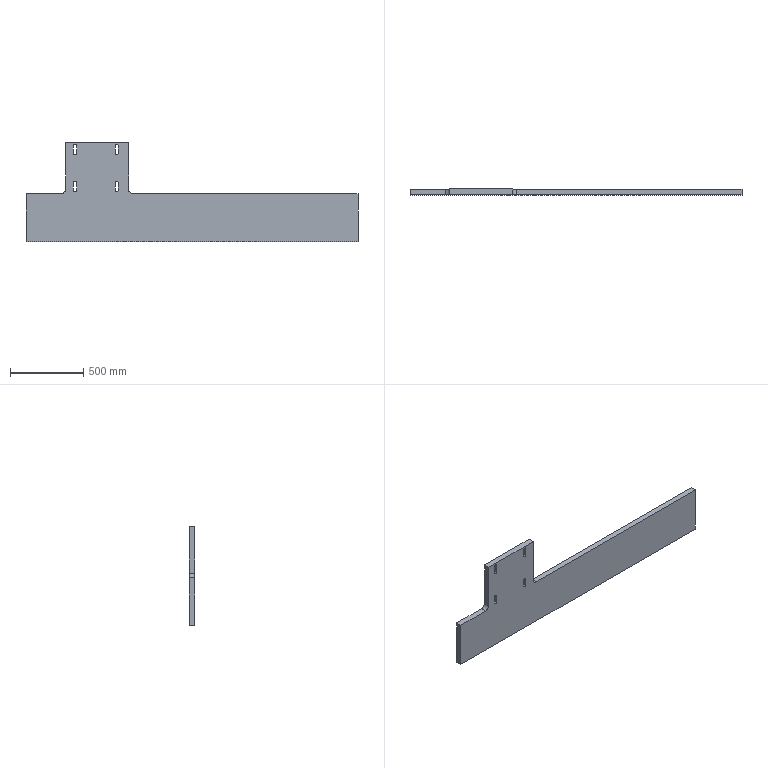Part | SolidWorks | features Cut 1, Extrusion 1, Fillet 1, ICE 1 | 1 solid | 32 faces | box 2266 x 40 x 677.5 mm | volume 35483230 mm3 | plane 18 | cylinder 14 | commonest cylinder face diameters 22 x12 60 x2
STEP:
#1=CARTESIAN_POINT('',(-514.,0.,500.75));
#2=VERTEX_POINT('',#1);
#3=CARTESIAN_POINT('',(-503.,0.,489.75));
#4=VERTEX_POINT('',#3);
#5=CARTESIAN_POINT('',(-514.,0.,489.75));
#6=DIRECTION('',(0.,1.,0.));
#7=DIRECTION('',(0.,0.,1.));
#8=AXIS2_PLACEMENT_3D('',#5,#6,#7);
#9=CIRCLE('',#8,11.);
#10=EDGE_CURVE('',#2,#4,#9,.T.);
#11=ORIENTED_EDGE('',*,*,#10,.F.);
#12=CARTESIAN_POINT('',(-514.,40.,500.75));
#13=VERTEX_POINT('',#12);
#14=CARTESIAN_POINT('',(-514.,0.,500.75));
#15=DIRECTION('',(0.,1.,0.));
#16=VECTOR('',#15,1000.);
#17=LINE('',#14,#16);
#18=EDGE_CURVE('',#2,#13,#17,.T.);
#19=ORIENTED_EDGE('',*,*,#18,.T.);
#20=CARTESIAN_POINT('',(-503.,40.,489.75));
#21=VERTEX_POINT('',#20);
#22=CARTESIAN_POINT('',(-514.,40.,489.75));
#23=DIRECTION('',(0.,1.,0.));
#24=DIRECTION('',(0.,0.,1.));
#25=AXIS2_PLACEMENT_3D('',#22,#23,#24);
#26=CIRCLE('',#25,11.);
#27=EDGE_CURVE('',#13,#21,#26,.T.);
#28=ORIENTED_EDGE('',*,*,#27,.T.);
#29=CARTESIAN_POINT('',(-503.,0.,489.75));
#30=DIRECTION('',(0.,1.,0.));
#31=VECTOR('',#30,1000.);
#32=LINE('',#29,#31);
#33=EDGE_CURVE('',#4,#21,#32,.T.);
#34=ORIENTED_EDGE('',*,*,#33,.F.);
#35=EDGE_LOOP('',(#11,#19,#28,#34));
#36=FACE_OUTER_BOUND('',#35,.T.);
#37=CARTESIAN_POINT('',(-514.,0.,489.75));
#38=DIRECTION('',(0.,1.,0.));
#39=DIRECTION('',(0.,0.,1.));
#40=AXIS2_PLACEMENT_3D('',#37,#38,#39);
#41=CYLINDRICAL_SURFACE('',#40,11.);
#42=ADVANCED_FACE('',(#36),#41,.F.);
#43=CARTESIAN_POINT('',(-798.,0.,248.75));
#44=VERTEX_POINT('',#43);
#45=CARTESIAN_POINT('',(-787.,0.,237.75));
#46=VERTEX_POINT('',#45);
#47=CARTESIAN_POINT('',(-798.,0.,237.75));
#48=DIRECTION('',(0.,1.,0.));
#49=DIRECTION('',(0.,0.,1.));
#50=AXIS2_PLACEMENT_3D('',#47,#48,#49);
#51=CIRCLE('',#50,11.);
#52=EDGE_CURVE('',#44,#46,#51,.T.);
#53=ORIENTED_EDGE('',*,*,#52,.F.);
#54=CARTESIAN_POINT('',(-798.,40.,248.75));
#55=VERTEX_POINT('',#54);
#56=CARTESIAN_POINT('',(-798.,0.,248.75));
#57=DIRECTION('',(0.,1.,0.));
#58=VECTOR('',#57,1000.);
#59=LINE('',#56,#58);
#60=EDGE_CURVE('',#44,#55,#59,.T.);
#61=ORIENTED_EDGE('',*,*,#60,.T.);
#62=CARTESIAN_POINT('',(-787.,40.,237.75));
#63=VERTEX_POINT('',#62);
#64=CARTESIAN_POINT('',(-798.,40.,237.75));
#65=DIRECTION('',(0.,1.,0.));
#66=DIRECTION('',(0.,0.,1.));
#67=AXIS2_PLACEMENT_3D('',#64,#65,#66);
#68=CIRCLE('',#67,11.);
#69=EDGE_CURVE('',#55,#63,#68,.T.);
#70=ORIENTED_EDGE('',*,*,#69,.T.);
#71=CARTESIAN_POINT('',(-787.,0.,237.75));
#72=DIRECTION('',(0.,1.,0.));
#73=VECTOR('',#72,1000.);
#74=LINE('',#71,#73);
#75=EDGE_CURVE('',#46,#63,#74,.T.);
#76=ORIENTED_EDGE('',*,*,#75,.F.);
#77=EDGE_LOOP('',(#53,#61,#70,#76));
#78=FACE_OUTER_BOUND('',#77,.T.);
#79=CARTESIAN_POINT('',(-798.,0.,237.75));
#80=DIRECTION('',(0.,1.,0.));
#81=DIRECTION('',(0.,0.,1.));
#82=AXIS2_PLACEMENT_3D('',#79,#80,#81);
#83=CYLINDRICAL_SURFACE('',#82,11.);
#84=ADVANCED_FACE('',(#78),#83,.F.);
#85=CARTESIAN_POINT('',(-798.,0.,500.75));
#86=VERTEX_POINT('',#85);
#87=CARTESIAN_POINT('',(-787.,0.,489.75));
#88=VERTEX_POINT('',#87);
#89=CARTESIAN_POINT('',(-798.,0.,489.75));
#90=DIRECTION('',(0.,1.,0.));
#91=DIRECTION('',(0.,0.,1.));
#92=AXIS2_PLACEMENT_3D('',#89,#90,#91);
#93=CIRCLE('',#92,11.);
#94=EDGE_CURVE('',#86,#88,#93,.T.);
#95=ORIENTED_EDGE('',*,*,#94,.F.);
#96=CARTESIAN_POINT('',(-798.,40.,500.75));
#97=VERTEX_POINT('',#96);
#98=CARTESIAN_POINT('',(-798.,0.,500.75));
#99=DIRECTION('',(0.,1.,0.));
#100=VECTOR('',#99,1000.);
#101=LINE('',#98,#100);
#102=EDGE_CURVE('',#86,#97,#101,.T.);
#103=ORIENTED_EDGE('',*,*,#102,.T.);
#104=CARTESIAN_POINT('',(-787.,40.,489.75));
#105=VERTEX_POINT('',#104);
#106=CARTESIAN_POINT('',(-798.,40.,489.75));
#107=DIRECTION('',(0.,1.,0.));
#108=DIRECTION('',(0.,0.,1.));
#109=AXIS2_PLACEMENT_3D('',#106,#107,#108);
#110=CIRCLE('',#109,11.);
#111=EDGE_CURVE('',#97,#105,#110,.T.);
#112=ORIENTED_EDGE('',*,*,#111,.T.);
#113=CARTESIAN_POINT('',(-787.,0.,489.75));
#114=DIRECTION('',(0.,1.,0.));
#115=VECTOR('',#114,1000.);
#116=LINE('',#113,#115);
#117=EDGE_CURVE('',#88,#105,#116,.T.);
#118=ORIENTED_EDGE('',*,*,#117,.F.);
#119=EDGE_LOOP('',(#95,#103,#112,#118));
#120=FACE_OUTER_BOUND('',#119,.T.);
#121=CARTESIAN_POINT('',(-798.,0.,489.75));
#122=DIRECTION('',(0.,1.,0.));
#123=DIRECTION('',(0.,0.,1.));
#124=AXIS2_PLACEMENT_3D('',#121,#122,#123);
#125=CYLINDRICAL_SURFACE('',#124,11.);
#126=ADVANCED_FACE('',(#120),#125,.F.);
#127=CARTESIAN_POINT('',(-514.,0.,248.75));
#128=VERTEX_POINT('',#127);
#129=CARTESIAN_POINT('',(-503.,0.,237.75));
#130=VERTEX_POINT('',#129);
#131=CARTESIAN_POINT('',(-514.,0.,237.75));
#132=DIRECTION('',(0.,1.,0.));
#133=DIRECTION('',(0.,0.,1.));
#134=AXIS2_PLACEMENT_3D('',#131,#132,#133);
#135=CIRCLE('',#134,11.);
#136=EDGE_CURVE('',#128,#130,#135,.T.);
#137=ORIENTED_EDGE('',*,*,#136,.F.);
#138=CARTESIAN_POINT('',(-514.,40.,248.75));
#139=VERTEX_POINT('',#138);
#140=CARTESIAN_POINT('',(-514.,0.,248.75));
#141=DIRECTION('',(0.,1.,0.));
#142=VECTOR('',#141,1000.);
#143=LINE('',#140,#142);
#144=EDGE_CURVE('',#128,#139,#143,.T.);
#145=ORIENTED_EDGE('',*,*,#144,.T.);
#146=CARTESIAN_POINT('',(-503.,40.,237.75));
#147=VERTEX_POINT('',#146);
#148=CARTESIAN_POINT('',(-514.,40.,237.75));
#149=DIRECTION('',(0.,1.,0.));
#150=DIRECTION('',(0.,0.,1.));
#151=AXIS2_PLACEMENT_3D('',#148,#149,#150);
#152=CIRCLE('',#151,11.);
#153=EDGE_CURVE('',#139,#147,#152,.T.);
#154=ORIENTED_EDGE('',*,*,#153,.T.);
#155=CARTESIAN_POINT('',(-503.,0.,237.75));
#156=DIRECTION('',(0.,1.,0.));
#157=VECTOR('',#156,1000.);
#158=LINE('',#155,#157);
#159=EDGE_CURVE('',#130,#147,#158,.T.);
#160=ORIENTED_EDGE('',*,*,#159,.F.);
#161=EDGE_LOOP('',(#137,#145,#154,#160));
#162=FACE_OUTER_BOUND('',#161,.T.);
#163=CARTESIAN_POINT('',(-514.,0.,237.75));
#164=DIRECTION('',(0.,1.,0.));
#165=DIRECTION('',(0.,0.,1.));
#166=AXIS2_PLACEMENT_3D('',#163,#164,#165);
#167=CYLINDRICAL_SURFACE('',#166,11.);
#168=ADVANCED_FACE('',(#162),#167,.F.);
#169=CARTESIAN_POINT('',(-403.,40.,163.75));
#170=VERTEX_POINT('',#169);
#171=CARTESIAN_POINT('',(1133.,40.,163.75));
#172=VERTEX_POINT('',#171);
#173=CARTESIAN_POINT('',(-1133.,40.,163.75));
#174=DIRECTION('',(1.,0.,0.));
#175=VECTOR('',#174,1000.);
#176=LINE('',#173,#175);
#177=EDGE_CURVE('',#170,#172,#176,.T.);
#178=ORIENTED_EDGE('',*,*,#177,.F.);
#179=CARTESIAN_POINT('',(-403.,0.,163.75));
#180=VERTEX_POINT('',#179);
#181=CARTESIAN_POINT('',(-403.,40.,163.75));
#182=DIRECTION('',(0.,-1.,0.));
#183=VECTOR('',#182,1000.);
#184=LINE('',#181,#183);
#185=EDGE_CURVE('',#170,#180,#184,.T.);
#186=ORIENTED_EDGE('',*,*,#185,.T.);
#187=CARTESIAN_POINT('',(1133.,0.,163.75));
#188=VERTEX_POINT('',#187);
#189=CARTESIAN_POINT('',(-1133.,0.,163.75));
#190=DIRECTION('',(1.,0.,0.));
#191=VECTOR('',#190,1000.);
#192=LINE('',#189,#191);
#193=EDGE_CURVE('',#180,#188,#192,.T.);
#194=ORIENTED_EDGE('',*,*,#193,.T.);
#195=CARTESIAN_POINT('',(1133.,40.,163.75));
#196=DIRECTION('',(0.,-1.,0.));
#197=VECTOR('',#196,1000.);
#198=LINE('',#195,#197);
#199=EDGE_CURVE('',#172,#188,#198,.T.);
#200=ORIENTED_EDGE('',*,*,#199,.F.);
#201=EDGE_LOOP('',(#178,#186,#194,#200));
#202=FACE_OUTER_BOUND('',#201,.T.);
#203=CARTESIAN_POINT('',(-1133.,40.,163.75));
#204=DIRECTION('',(0.,0.,-1.));
#205=DIRECTION('',(-1.,0.,0.));
#206=AXIS2_PLACEMENT_3D('',#203,#204,#205);
#207=PLANE('',#206);
#208=ADVANCED_FACE('',(#202),#207,.F.);
#209=CARTESIAN_POINT('',(1133.,0.,-163.75));
#210=VERTEX_POINT('',#209);
#211=CARTESIAN_POINT('',(1133.,0.,163.75));
#212=DIRECTION('',(0.,0.,-1.));
#213=VECTOR('',#212,1000.);
#214=LINE('',#211,#213);
#215=EDGE_CURVE('',#188,#210,#214,.T.);
#216=ORIENTED_EDGE('',*,*,#215,.T.);
#217=CARTESIAN_POINT('',(1133.,40.,-163.75));
#218=VERTEX_POINT('',#217);
#219=CARTESIAN_POINT('',(1133.,40.,-163.75));
#220=DIRECTION('',(0.,-1.,0.));
#221=VECTOR('',#220,1000.);
#222=LINE('',#219,#221);
#223=EDGE_CURVE('',#218,#210,#222,.T.);
#224=ORIENTED_EDGE('',*,*,#223,.F.);
#225=CARTESIAN_POINT('',(1133.,40.,163.75));
#226=DIRECTION('',(0.,0.,-1.));
#227=VECTOR('',#226,1000.);
#228=LINE('',#225,#227);
#229=EDGE_CURVE('',#172,#218,#228,.T.);
#230=ORIENTED_EDGE('',*,*,#229,.F.);
#231=ORIENTED_EDGE('',*,*,#199,.T.);
#232=EDGE_LOOP('',(#216,#224,#230,#231));
#233=FACE_OUTER_BOUND('',#232,.T.);
#234=CARTESIAN_POINT('',(1133.,40.,163.75));
#235=DIRECTION('',(-1.,0.,0.));
#236=DIRECTION('',(0.,0.,1.));
#237=AXIS2_PLACEMENT_3D('',#234,#235,#236);
#238=PLANE('',#237);
#239=ADVANCED_FACE('',(#233),#238,.F.);
#240=CARTESIAN_POINT('',(-1133.,0.,-163.75));
#241=VERTEX_POINT('',#240);
#242=CARTESIAN_POINT('',(-1133.,0.,-163.75));
#243=DIRECTION('',(-1.,0.,0.));
#244=VECTOR('',#243,1000.);
#245=LINE('',#242,#244);
#246=EDGE_CURVE('',#210,#241,#245,.T.);
#247=ORIENTED_EDGE('',*,*,#246,.T.);
#248=CARTESIAN_POINT('',(-1133.,40.,-163.75));
#249=VERTEX_POINT('',#248);
#250=CARTESIAN_POINT('',(-1133.,40.,-163.75));
#251=DIRECTION('',(0.,-1.,0.));
#252=VECTOR('',#251,1000.);
#253=LINE('',#250,#252);
#254=EDGE_CURVE('',#249,#241,#253,.T.);
#255=ORIENTED_EDGE('',*,*,#254,.F.);
#256=CARTESIAN_POINT('',(-1133.,40.,-163.75));
#257=DIRECTION('',(-1.,0.,0.));
#258=VECTOR('',#257,1000.);
#259=LINE('',#256,#258);
#260=EDGE_CURVE('',#218,#249,#259,.T.);
#261=ORIENTED_EDGE('',*,*,#260,.F.);
#262=ORIENTED_EDGE('',*,*,#223,.T.);
#263=EDGE_LOOP('',(#247,#255,#261,#262));
#264=FACE_OUTER_BOUND('',#263,.T.);
#265=CARTESIAN_POINT('',(-1133.,40.,-163.75));
#266=DIRECTION('',(0.,0.,1.));
#267=DIRECTION('',(1.,0.,0.));
#268=AXIS2_PLACEMENT_3D('',#265,#266,#267);
#269=PLANE('',#268);
#270=ADVANCED_FACE('',(#264),#269,.F.);
#271=CARTESIAN_POINT('',(-1133.,0.,163.75));
#272=VERTEX_POINT('',#271);
#273=CARTESIAN_POINT('',(-1133.,0.,163.75));
#274=DIRECTION('',(0.,0.,1.));
#275=VECTOR('',#274,1000.);
#276=LINE('',#273,#275);
#277=EDGE_CURVE('',#241,#272,#276,.T.);
#278=ORIENTED_EDGE('',*,*,#277,.T.);
#279=CARTESIAN_POINT('',(-1133.,40.,163.75));
#280=VERTEX_POINT('',#279);
#281=CARTESIAN_POINT('',(-1133.,40.,163.75));
#282=DIRECTION('',(0.,-1.,0.));
#283=VECTOR('',#282,1000.);
#284=LINE('',#281,#283);
#285=EDGE_CURVE('',#280,#272,#284,.T.);
#286=ORIENTED_EDGE('',*,*,#285,.F.);
#287=CARTESIAN_POINT('',(-1133.,40.,163.75));
#288=DIRECTION('',(0.,0.,1.));
#289=VECTOR('',#288,1000.);
#290=LINE('',#287,#289);
#291=EDGE_CURVE('',#249,#280,#290,.T.);
#292=ORIENTED_EDGE('',*,*,#291,.F.);
#293=ORIENTED_EDGE('',*,*,#254,.T.);
#294=EDGE_LOOP('',(#278,#286,#292,#293));
#295=FACE_OUTER_BOUND('',#294,.T.);
#296=CARTESIAN_POINT('',(-1133.,40.,163.75));
#297=DIRECTION('',(1.,0.,0.));
#298=DIRECTION('',(0.,0.,-1.));
#299=AXIS2_PLACEMENT_3D('',#296,#297,#298);
#300=PLANE('',#299);
#301=ADVANCED_FACE('',(#295),#300,.F.);
#302=CARTESIAN_POINT('',(-893.,0.,163.75));
#303=VERTEX_POINT('',#302);
#304=CARTESIAN_POINT('',(-1133.,0.,163.75));
#305=DIRECTION('',(1.,0.,0.));
#306=VECTOR('',#305,1000.);
#307=LINE('',#304,#306);
#308=EDGE_CURVE('',#272,#303,#307,.T.);
#309=ORIENTED_EDGE('',*,*,#308,.T.);
#310=CARTESIAN_POINT('',(-893.,40.,163.75));
#311=VERTEX_POINT('',#310);
#312=CARTESIAN_POINT('',(-893.,40.,163.75));
#313=DIRECTION('',(0.,1.,0.));
#314=VECTOR('',#313,1000.);
#315=LINE('',#312,#314);
#316=EDGE_CURVE('',#303,#311,#315,.T.);
#317=ORIENTED_EDGE('',*,*,#316,.T.);
#318=CARTESIAN_POINT('',(-1133.,40.,163.75));
#319=DIRECTION('',(1.,0.,0.));
#320=VECTOR('',#319,1000.);
#321=LINE('',#318,#320);
#322=EDGE_CURVE('',#280,#311,#321,.T.);
#323=ORIENTED_EDGE('',*,*,#322,.F.);
#324=ORIENTED_EDGE('',*,*,#285,.T.);
#325=EDGE_LOOP('',(#309,#317,#323,#324));
#326=FACE_OUTER_BOUND('',#325,.T.);
#327=CARTESIAN_POINT('',(-1133.,40.,163.75));
#328=DIRECTION('',(0.,0.,-1.));
#329=DIRECTION('',(-1.,0.,0.));
#330=AXIS2_PLACEMENT_3D('',#327,#328,#329);
#331=PLANE('',#330);
#332=ADVANCED_FACE('',(#326),#331,.F.);
#333=CARTESIAN_POINT('',(-525.,40.,439.75));
#334=VERTEX_POINT('',#333);
#335=CARTESIAN_POINT('',(-525.,40.,489.75));
#336=VERTEX_POINT('',#335);
#337=CARTESIAN_POINT('',(-525.,40.,439.75));
#338=DIRECTION('',(0.,0.,1.));
#339=VECTOR('',#338,1000.);
#340=LINE('',#337,#339);
#341=EDGE_CURVE('',#334,#336,#340,.T.);
#342=ORIENTED_EDGE('',*,*,#341,.F.);
#343=CARTESIAN_POINT('',(-503.,40.,439.75));
#344=VERTEX_POINT('',#343);
#345=CARTESIAN_POINT('',(-514.,40.,439.75));
#346=DIRECTION('',(0.,1.,0.));
#347=DIRECTION('',(0.,0.,1.));
#348=AXIS2_PLACEMENT_3D('',#345,#346,#347);
#349=CIRCLE('',#348,11.);
#350=EDGE_CURVE('',#344,#334,#349,.T.);
#351=ORIENTED_EDGE('',*,*,#350,.F.);
#352=CARTESIAN_POINT('',(-503.,40.,439.75));
#353=DIRECTION('',(0.,0.,-1.));
#354=VECTOR('',#353,1000.);
#355=LINE('',#352,#354);
#356=EDGE_CURVE('',#21,#344,#355,.T.);
#357=ORIENTED_EDGE('',*,*,#356,.F.);
#358=ORIENTED_EDGE('',*,*,#27,.F.);
#359=CARTESIAN_POINT('',(-514.,40.,489.75));
#360=DIRECTION('',(0.,1.,0.));
#361=DIRECTION('',(0.,0.,1.));
#362=AXIS2_PLACEMENT_3D('',#359,#360,#361);
#363=CIRCLE('',#362,11.);
#364=EDGE_CURVE('',#336,#13,#363,.T.);
#365=ORIENTED_EDGE('',*,*,#364,.F.);
#366=EDGE_LOOP('',(#342,#351,#357,#358,#365));
#367=FACE_BOUND('',#366,.T.);
#368=CARTESIAN_POINT('',(-809.,40.,187.75));
#369=VERTEX_POINT('',#368);
#370=CARTESIAN_POINT('',(-809.,40.,237.75));
#371=VERTEX_POINT('',#370);
#372=CARTESIAN_POINT('',(-809.,40.,187.75));
#373=DIRECTION('',(0.,0.,1.));
#374=VECTOR('',#373,1000.);
#375=LINE('',#372,#374);
#376=EDGE_CURVE('',#369,#371,#375,.T.);
#377=ORIENTED_EDGE('',*,*,#376,.F.);
#378=CARTESIAN_POINT('',(-787.,40.,187.75));
#379=VERTEX_POINT('',#378);
#380=CARTESIAN_POINT('',(-798.,40.,187.75));
#381=DIRECTION('',(0.,1.,0.));
#382=DIRECTION('',(0.,0.,1.));
#383=AXIS2_PLACEMENT_3D('',#380,#381,#382);
#384=CIRCLE('',#383,11.);
#385=EDGE_CURVE('',#379,#369,#384,.T.);
#386=ORIENTED_EDGE('',*,*,#385,.F.);
#387=CARTESIAN_POINT('',(-787.,40.,187.75));
#388=DIRECTION('',(0.,0.,-1.));
#389=VECTOR('',#388,1000.);
#390=LINE('',#387,#389);
#391=EDGE_CURVE('',#63,#379,#390,.T.);
#392=ORIENTED_EDGE('',*,*,#391,.F.);
#393=ORIENTED_EDGE('',*,*,#69,.F.);
#394=CARTESIAN_POINT('',(-798.,40.,237.75));
#395=DIRECTION('',(0.,1.,0.));
#396=DIRECTION('',(0.,0.,1.));
#397=AXIS2_PLACEMENT_3D('',#394,#395,#396);
#398=CIRCLE('',#397,11.);
#399=EDGE_CURVE('',#371,#55,#398,.T.);
#400=ORIENTED_EDGE('',*,*,#399,.F.);
#401=EDGE_LOOP('',(#377,#386,#392,#393,#400));
#402=FACE_BOUND('',#401,.T.);
#403=CARTESIAN_POINT('',(-809.,40.,439.75));
#404=VERTEX_POINT('',#403);
#405=CARTESIAN_POINT('',(-809.,40.,489.75));
#406=VERTEX_POINT('',#405);
#407=CARTESIAN_POINT('',(-809.,40.,439.75));
#408=DIRECTION('',(0.,0.,1.));
#409=VECTOR('',#408,1000.);
#410=LINE('',#407,#409);
#411=EDGE_CURVE('',#404,#406,#410,.T.);
#412=ORIENTED_EDGE('',*,*,#411,.F.);
#413=CARTESIAN_POINT('',(-787.,40.,439.75));
#414=VERTEX_POINT('',#413);
#415=CARTESIAN_POINT('',(-798.,40.,439.75));
#416=DIRECTION('',(0.,1.,0.));
#417=DIRECTION('',(0.,0.,1.));
#418=AXIS2_PLACEMENT_3D('',#415,#416,#417);
#419=CIRCLE('',#418,11.);
#420=EDGE_CURVE('',#414,#404,#419,.T.);
#421=ORIENTED_EDGE('',*,*,#420,.F.);
#422=CARTESIAN_POINT('',(-787.,40.,439.75));
#423=DIRECTION('',(0.,0.,-1.));
#424=VECTOR('',#423,1000.);
#425=LINE('',#422,#424);
#426=EDGE_CURVE('',#105,#414,#425,.T.);
#427=ORIENTED_EDGE('',*,*,#426,.F.);
#428=ORIENTED_EDGE('',*,*,#111,.F.);
#429=CARTESIAN_POINT('',(-798.,40.,489.75));
#430=DIRECTION('',(0.,1.,0.));
#431=DIRECTION('',(0.,0.,1.));
#432=AXIS2_PLACEMENT_3D('',#429,#430,#431);
#433=CIRCLE('',#432,11.);
#434=EDGE_CURVE('',#406,#97,#433,.T.);
#435=ORIENTED_EDGE('',*,*,#434,.F.);
#436=EDGE_LOOP('',(#412,#421,#427,#428,#435));
#437=FACE_BOUND('',#436,.T.);
#438=CARTESIAN_POINT('',(-525.,40.,187.75));
#439=VERTEX_POINT('',#438);
#440=CARTESIAN_POINT('',(-525.,40.,237.75));
#441=VERTEX_POINT('',#440);
#442=CARTESIAN_POINT('',(-525.,40.,187.75));
#443=DIRECTION('',(0.,0.,1.));
#444=VECTOR('',#443,1000.);
#445=LINE('',#442,#444);
#446=EDGE_CURVE('',#439,#441,#445,.T.);
#447=ORIENTED_EDGE('',*,*,#446,.F.);
#448=CARTESIAN_POINT('',(-503.,40.,187.75));
#449=VERTEX_POINT('',#448);
#450=CARTESIAN_POINT('',(-514.,40.,187.75));
#451=DIRECTION('',(0.,1.,0.));
#452=DIRECTION('',(0.,0.,1.));
#453=AXIS2_PLACEMENT_3D('',#450,#451,#452);
#454=CIRCLE('',#453,11.);
#455=EDGE_CURVE('',#449,#439,#454,.T.);
#456=ORIENTED_EDGE('',*,*,#455,.F.);
#457=CARTESIAN_POINT('',(-503.,40.,187.75));
#458=DIRECTION('',(0.,0.,-1.));
#459=VECTOR('',#458,1000.);
#460=LINE('',#457,#459);
#461=EDGE_CURVE('',#147,#449,#460,.T.);
#462=ORIENTED_EDGE('',*,*,#461,.F.);
#463=ORIENTED_EDGE('',*,*,#153,.F.);
#464=CARTESIAN_POINT('',(-514.,40.,237.75));
#465=DIRECTION('',(0.,1.,0.));
#466=DIRECTION('',(0.,0.,1.));
#467=AXIS2_PLACEMENT_3D('',#464,#465,#466);
#468=CIRCLE('',#467,11.);
#469=EDGE_CURVE('',#441,#139,#468,.T.);
#470=ORIENTED_EDGE('',*,*,#469,.F.);
#471=EDGE_LOOP('',(#447,#456,#462,#463,#470));
#472=FACE_BOUND('',#471,.T.);
#473=ORIENTED_EDGE('',*,*,#229,.T.);
#474=ORIENTED_EDGE('',*,*,#260,.T.);
#475=ORIENTED_EDGE('',*,*,#291,.T.);
#476=ORIENTED_EDGE('',*,*,#322,.T.);
#477=CARTESIAN_POINT('',(-863.,40.,193.75));
#478=VERTEX_POINT('',#477);
#479=CARTESIAN_POINT('',(-893.,40.,193.75));
#480=DIRECTION('',(0.,-1.,0.));
#481=DIRECTION('',(0.,0.,-1.));
#482=AXIS2_PLACEMENT_3D('',#479,#480,#481);
#483=CIRCLE('',#482,30.);
#484=EDGE_CURVE('',#311,#478,#483,.T.);
#485=ORIENTED_EDGE('',*,*,#484,.T.);
#486=CARTESIAN_POINT('',(-863.,40.,513.75));
#487=VERTEX_POINT('',#486);
#488=CARTESIAN_POINT('',(-863.,40.,163.75));
#489=DIRECTION('',(0.,0.,1.));
#490=VECTOR('',#489,1000.);
#491=LINE('',#488,#490);
#492=EDGE_CURVE('',#478,#487,#491,.T.);
#493=ORIENTED_EDGE('',*,*,#492,.T.);
#494=CARTESIAN_POINT('',(-433.,40.,513.75));
#495=VERTEX_POINT('',#494);
#496=CARTESIAN_POINT('',(-433.,40.,513.75));
#497=DIRECTION('',(1.,0.,0.));
#498=VECTOR('',#497,1000.);
#499=LINE('',#496,#498);
#500=EDGE_CURVE('',#487,#495,#499,.T.);
#501=ORIENTED_EDGE('',*,*,#500,.T.);
#502=CARTESIAN_POINT('',(-433.,40.,193.75));
#503=VERTEX_POINT('',#502);
#504=CARTESIAN_POINT('',(-433.,40.,163.75));
#505=DIRECTION('',(0.,0.,-1.));
#506=VECTOR('',#505,1000.);
#507=LINE('',#504,#506);
#508=EDGE_CURVE('',#495,#503,#507,.T.);
#509=ORIENTED_EDGE('',*,*,#508,.T.);
#510=CARTESIAN_POINT('',(-403.,40.,193.75));
#511=DIRECTION('',(0.,-1.,0.));
#512=DIRECTION('',(0.,0.,-1.));
#513=AXIS2_PLACEMENT_3D('',#510,#511,#512);
#514=CIRCLE('',#513,30.);
#515=EDGE_CURVE('',#503,#170,#514,.T.);
#516=ORIENTED_EDGE('',*,*,#515,.T.);
#517=ORIENTED_EDGE('',*,*,#177,.T.);
#518=EDGE_LOOP('',(#473,#474,#475,#476,#485,#493,#501,#509,#516,#517));
#519=FACE_OUTER_BOUND('',#518,.T.);
#520=CARTESIAN_POINT('',(0.,40.,0.));
#521=DIRECTION('',(0.,-1.,0.));
#522=DIRECTION('',(0.,0.,-1.));
#523=AXIS2_PLACEMENT_3D('',#520,#521,#522);
#524=PLANE('',#523);
#525=ADVANCED_FACE('',(#367,#402,#437,#472,#519),#524,.F.);
#526=CARTESIAN_POINT('',(-503.,0.,439.75));
#527=VERTEX_POINT('',#526);
#528=CARTESIAN_POINT('',(-525.,0.,439.75));
#529=VERTEX_POINT('',#528);
#530=CARTESIAN_POINT('',(-514.,0.,439.75));
#531=DIRECTION('',(0.,1.,0.));
#532=DIRECTION('',(0.,0.,1.));
#533=AXIS2_PLACEMENT_3D('',#530,#531,#532);
#534=CIRCLE('',#533,11.);
#535=EDGE_CURVE('',#527,#529,#534,.T.);
#536=ORIENTED_EDGE('',*,*,#535,.T.);
#537=CARTESIAN_POINT('',(-525.,0.,489.75));
#538=VERTEX_POINT('',#537);
#539=CARTESIAN_POINT('',(-525.,0.,439.75));
#540=DIRECTION('',(0.,0.,1.));
#541=VECTOR('',#540,1000.);
#542=LINE('',#539,#541);
#543=EDGE_CURVE('',#529,#538,#542,.T.);
#544=ORIENTED_EDGE('',*,*,#543,.T.);
#545=CARTESIAN_POINT('',(-514.,0.,489.75));
#546=DIRECTION('',(0.,1.,0.));
#547=DIRECTION('',(0.,0.,1.));
#548=AXIS2_PLACEMENT_3D('',#545,#546,#547);
#549=CIRCLE('',#548,11.);
#550=EDGE_CURVE('',#538,#2,#549,.T.);
#551=ORIENTED_EDGE('',*,*,#550,.T.);
#552=ORIENTED_EDGE('',*,*,#10,.T.);
#553=CARTESIAN_POINT('',(-503.,0.,439.75));
#554=DIRECTION('',(0.,0.,-1.));
#555=VECTOR('',#554,1000.);
#556=LINE('',#553,#555);
#557=EDGE_CURVE('',#4,#527,#556,.T.);
#558=ORIENTED_EDGE('',*,*,#557,.T.);
#559=EDGE_LOOP('',(#536,#544,#551,#552,#558));
#560=FACE_BOUND('',#559,.T.);
#561=CARTESIAN_POINT('',(-787.,0.,187.75));
#562=VERTEX_POINT('',#561);
#563=CARTESIAN_POINT('',(-809.,0.,187.75));
#564=VERTEX_POINT('',#563);
#565=CARTESIAN_POINT('',(-798.,0.,187.75));
#566=DIRECTION('',(0.,1.,0.));
#567=DIRECTION('',(0.,0.,1.));
#568=AXIS2_PLACEMENT_3D('',#565,#566,#567);
#569=CIRCLE('',#568,11.);
#570=EDGE_CURVE('',#562,#564,#569,.T.);
#571=ORIENTED_EDGE('',*,*,#570,.T.);
#572=CARTESIAN_POINT('',(-809.,0.,237.75));
#573=VERTEX_POINT('',#572);
#574=CARTESIAN_POINT('',(-809.,0.,187.75));
#575=DIRECTION('',(0.,0.,1.));
#576=VECTOR('',#575,1000.);
#577=LINE('',#574,#576);
#578=EDGE_CURVE('',#564,#573,#577,.T.);
#579=ORIENTED_EDGE('',*,*,#578,.T.);
#580=CARTESIAN_POINT('',(-798.,0.,237.75));
#581=DIRECTION('',(0.,1.,0.));
#582=DIRECTION('',(0.,0.,1.));
#583=AXIS2_PLACEMENT_3D('',#580,#581,#582);
#584=CIRCLE('',#583,11.);
#585=EDGE_CURVE('',#573,#44,#584,.T.);
#586=ORIENTED_EDGE('',*,*,#585,.T.);
#587=ORIENTED_EDGE('',*,*,#52,.T.);
#588=CARTESIAN_POINT('',(-787.,0.,187.75));
#589=DIRECTION('',(0.,0.,-1.));
#590=VECTOR('',#589,1000.);
#591=LINE('',#588,#590);
#592=EDGE_CURVE('',#46,#562,#591,.T.);
#593=ORIENTED_EDGE('',*,*,#592,.T.);
#594=EDGE_LOOP('',(#571,#579,#586,#587,#593));
#595=FACE_BOUND('',#594,.T.);
#596=CARTESIAN_POINT('',(-787.,0.,439.75));
#597=VERTEX_POINT('',#596);
#598=CARTESIAN_POINT('',(-809.,0.,439.75));
#599=VERTEX_POINT('',#598);
#600=CARTESIAN_POINT('',(-798.,0.,439.75));
#601=DIRECTION('',(0.,1.,0.));
#602=DIRECTION('',(0.,0.,1.));
#603=AXIS2_PLACEMENT_3D('',#600,#601,#602);
#604=CIRCLE('',#603,11.);
#605=EDGE_CURVE('',#597,#599,#604,.T.);
#606=ORIENTED_EDGE('',*,*,#605,.T.);
#607=CARTESIAN_POINT('',(-809.,0.,489.75));
#608=VERTEX_POINT('',#607);
#609=CARTESIAN_POINT('',(-809.,0.,439.75));
#610=DIRECTION('',(0.,0.,1.));
#611=VECTOR('',#610,1000.);
#612=LINE('',#609,#611);
#613=EDGE_CURVE('',#599,#608,#612,.T.);
#614=ORIENTED_EDGE('',*,*,#613,.T.);
#615=CARTESIAN_POINT('',(-798.,0.,489.75));
#616=DIRECTION('',(0.,1.,0.));
#617=DIRECTION('',(0.,0.,1.));
#618=AXIS2_PLACEMENT_3D('',#615,#616,#617);
#619=CIRCLE('',#618,11.);
#620=EDGE_CURVE('',#608,#86,#619,.T.);
#621=ORIENTED_EDGE('',*,*,#620,.T.);
#622=ORIENTED_EDGE('',*,*,#94,.T.);
#623=CARTESIAN_POINT('',(-787.,0.,439.75));
#624=DIRECTION('',(0.,0.,-1.));
#625=VECTOR('',#624,1000.);
#626=LINE('',#623,#625);
#627=EDGE_CURVE('',#88,#597,#626,.T.);
#628=ORIENTED_EDGE('',*,*,#627,.T.);
#629=EDGE_LOOP('',(#606,#614,#621,#622,#628));
#630=FACE_BOUND('',#629,.T.);
#631=CARTESIAN_POINT('',(-503.,0.,187.75));
#632=VERTEX_POINT('',#631);
#633=CARTESIAN_POINT('',(-525.,0.,187.75));
#634=VERTEX_POINT('',#633);
#635=CARTESIAN_POINT('',(-514.,0.,187.75));
#636=DIRECTION('',(0.,1.,0.));
#637=DIRECTION('',(0.,0.,1.));
#638=AXIS2_PLACEMENT_3D('',#635,#636,#637);
#639=CIRCLE('',#638,11.);
#640=EDGE_CURVE('',#632,#634,#639,.T.);
#641=ORIENTED_EDGE('',*,*,#640,.T.);
#642=CARTESIAN_POINT('',(-525.,0.,237.75));
#643=VERTEX_POINT('',#642);
#644=CARTESIAN_POINT('',(-525.,0.,187.75));
#645=DIRECTION('',(0.,0.,1.));
#646=VECTOR('',#645,1000.);
#647=LINE('',#644,#646);
#648=EDGE_CURVE('',#634,#643,#647,.T.);
#649=ORIENTED_EDGE('',*,*,#648,.T.);
#650=CARTESIAN_POINT('',(-514.,0.,237.75));
#651=DIRECTION('',(0.,1.,0.));
#652=DIRECTION('',(0.,0.,1.));
#653=AXIS2_PLACEMENT_3D('',#650,#651,#652);
#654=CIRCLE('',#653,11.);
#655=EDGE_CURVE('',#643,#128,#654,.T.);
#656=ORIENTED_EDGE('',*,*,#655,.T.);
#657=ORIENTED_EDGE('',*,*,#136,.T.);
#658=CARTESIAN_POINT('',(-503.,0.,187.75));
#659=DIRECTION('',(0.,0.,-1.));
#660=VECTOR('',#659,1000.);
#661=LINE('',#658,#660);
#662=EDGE_CURVE('',#130,#632,#661,.T.);
#663=ORIENTED_EDGE('',*,*,#662,.T.);
#664=EDGE_LOOP('',(#641,#649,#656,#657,#663));
#665=FACE_BOUND('',#664,.T.);
#666=ORIENTED_EDGE('',*,*,#215,.F.);
#667=ORIENTED_EDGE('',*,*,#193,.F.);
#668=CARTESIAN_POINT('',(-433.,0.,193.75));
#669=VERTEX_POINT('',#668);
#670=CARTESIAN_POINT('',(-403.,0.,193.75));
#671=DIRECTION('',(0.,1.,0.));
#672=DIRECTION('',(0.,0.,-1.));
#673=AXIS2_PLACEMENT_3D('',#670,#671,#672);
#674=CIRCLE('',#673,30.);
#675=EDGE_CURVE('',#180,#669,#674,.T.);
#676=ORIENTED_EDGE('',*,*,#675,.T.);
#677=CARTESIAN_POINT('',(-433.,0.,513.75));
#678=VERTEX_POINT('',#677);
#679=CARTESIAN_POINT('',(-433.,0.,163.75));
#680=DIRECTION('',(0.,0.,-1.));
#681=VECTOR('',#680,1000.);
#682=LINE('',#679,#681);
#683=EDGE_CURVE('',#678,#669,#682,.T.);
#684=ORIENTED_EDGE('',*,*,#683,.F.);
#685=CARTESIAN_POINT('',(-863.,0.,513.75));
#686=VERTEX_POINT('',#685);
#687=CARTESIAN_POINT('',(-433.,0.,513.75));
#688=DIRECTION('',(1.,0.,0.));
#689=VECTOR('',#688,1000.);
#690=LINE('',#687,#689);
#691=EDGE_CURVE('',#686,#678,#690,.T.);
#692=ORIENTED_EDGE('',*,*,#691,.F.);
#693=CARTESIAN_POINT('',(-863.,0.,193.75));
#694=VERTEX_POINT('',#693);
#695=CARTESIAN_POINT('',(-863.,0.,163.75));
#696=DIRECTION('',(0.,0.,1.));
#697=VECTOR('',#696,1000.);
#698=LINE('',#695,#697);
#699=EDGE_CURVE('',#694,#686,#698,.T.);
#700=ORIENTED_EDGE('',*,*,#699,.F.);
#701=CARTESIAN_POINT('',(-893.,0.,193.75));
#702=DIRECTION('',(0.,1.,0.));
#703=DIRECTION('',(0.,0.,-1.));
#704=AXIS2_PLACEMENT_3D('',#701,#702,#703);
#705=CIRCLE('',#704,30.);
#706=EDGE_CURVE('',#694,#303,#705,.T.);
#707=ORIENTED_EDGE('',*,*,#706,.T.);
#708=ORIENTED_EDGE('',*,*,#308,.F.);
#709=ORIENTED_EDGE('',*,*,#277,.F.);
#710=ORIENTED_EDGE('',*,*,#246,.F.);
#711=EDGE_LOOP('',(#666,#667,#676,#684,#692,#700,#707,#708,#709,#710));
#712=FACE_OUTER_BOUND('',#711,.T.);
#713=CARTESIAN_POINT('',(0.,0.,0.));
#714=DIRECTION('',(0.,-1.,0.));
#715=DIRECTION('',(0.,0.,-1.));
#716=AXIS2_PLACEMENT_3D('',#713,#714,#715);
#717=PLANE('',#716);
#718=ADVANCED_FACE('',(#560,#595,#630,#665,#712),#717,.T.);
#719=ORIENTED_EDGE('',*,*,#683,.T.);
#720=CARTESIAN_POINT('',(-433.,0.,193.75));
#721=DIRECTION('',(0.,1.,0.));
#722=VECTOR('',#721,1000.);
#723=LINE('',#720,#722);
#724=EDGE_CURVE('',#669,#503,#723,.T.);
#725=ORIENTED_EDGE('',*,*,#724,.T.);
#726=ORIENTED_EDGE('',*,*,#508,.F.);
#727=CARTESIAN_POINT('',(-433.,0.,513.75));
#728=DIRECTION('',(0.,1.,0.));
#729=VECTOR('',#728,1000.);
#730=LINE('',#727,#729);
#731=EDGE_CURVE('',#678,#495,#730,.T.);
#732=ORIENTED_EDGE('',*,*,#731,.F.);
#733=EDGE_LOOP('',(#719,#725,#726,#732));
#734=FACE_OUTER_BOUND('',#733,.T.);
#735=CARTESIAN_POINT('',(-433.,0.,163.75));
#736=DIRECTION('',(1.,0.,0.));
#737=DIRECTION('',(0.,0.,-1.));
#738=AXIS2_PLACEMENT_3D('',#735,#736,#737);
#739=PLANE('',#738);
#740=ADVANCED_FACE('',(#734),#739,.T.);
#741=ORIENTED_EDGE('',*,*,#500,.F.);
#742=CARTESIAN_POINT('',(-863.,0.,513.75));
#743=DIRECTION('',(0.,1.,0.));
#744=VECTOR('',#743,1000.);
#745=LINE('',#742,#744);
#746=EDGE_CURVE('',#686,#487,#745,.T.);
#747=ORIENTED_EDGE('',*,*,#746,.F.);
#748=ORIENTED_EDGE('',*,*,#691,.T.);
#749=ORIENTED_EDGE('',*,*,#731,.T.);
#750=EDGE_LOOP('',(#741,#747,#748,#749));
#751=FACE_OUTER_BOUND('',#750,.T.);
#752=CARTESIAN_POINT('',(-433.,0.,513.75));
#753=DIRECTION('',(0.,0.,1.));
#754=DIRECTION('',(1.,0.,0.));
#755=AXIS2_PLACEMENT_3D('',#752,#753,#754);
#756=PLANE('',#755);
#757=ADVANCED_FACE('',(#751),#756,.T.);
#758=ORIENTED_EDGE('',*,*,#492,.F.);
#759=CARTESIAN_POINT('',(-863.,0.,193.75));
#760=DIRECTION('',(0.,-1.,0.));
#761=VECTOR('',#760,1000.);
#762=LINE('',#759,#761);
#763=EDGE_CURVE('',#478,#694,#762,.T.);
#764=ORIENTED_EDGE('',*,*,#763,.T.);
#765=ORIENTED_EDGE('',*,*,#699,.T.);
#766=ORIENTED_EDGE('',*,*,#746,.T.);
#767=EDGE_LOOP('',(#758,#764,#765,#766));
#768=FACE_OUTER_BOUND('',#767,.T.);
#769=CARTESIAN_POINT('',(-863.,0.,163.75));
#770=DIRECTION('',(-1.,0.,0.));
#771=DIRECTION('',(0.,0.,1.));
#772=AXIS2_PLACEMENT_3D('',#769,#770,#771);
#773=PLANE('',#772);
#774=ADVANCED_FACE('',(#768),#773,.T.);
#775=ORIENTED_EDGE('',*,*,#455,.T.);
#776=CARTESIAN_POINT('',(-525.,0.,187.75));
#777=DIRECTION('',(0.,1.,0.));
#778=VECTOR('',#777,1000.);
#779=LINE('',#776,#778);
#780=EDGE_CURVE('',#634,#439,#779,.T.);
#781=ORIENTED_EDGE('',*,*,#780,.F.);
#782=ORIENTED_EDGE('',*,*,#640,.F.);
#783=CARTESIAN_POINT('',(-503.,0.,187.75));
#784=DIRECTION('',(0.,1.,0.));
#785=VECTOR('',#784,1000.);
#786=LINE('',#783,#785);
#787=EDGE_CURVE('',#632,#449,#786,.T.);
#788=ORIENTED_EDGE('',*,*,#787,.T.);
#789=EDGE_LOOP('',(#775,#781,#782,#788));
#790=FACE_OUTER_BOUND('',#789,.T.);
#791=CARTESIAN_POINT('',(-514.,0.,187.75));
#792=DIRECTION('',(0.,1.,0.));
#793=DIRECTION('',(0.,0.,1.));
#794=AXIS2_PLACEMENT_3D('',#791,#792,#793);
#795=CYLINDRICAL_SURFACE('',#794,11.);
#796=ADVANCED_FACE('',(#790),#795,.F.);
#797=ORIENTED_EDGE('',*,*,#461,.T.);
#798=ORIENTED_EDGE('',*,*,#787,.F.);
#799=ORIENTED_EDGE('',*,*,#662,.F.);
#800=ORIENTED_EDGE('',*,*,#159,.T.);
#801=EDGE_LOOP('',(#797,#798,#799,#800));
#802=FACE_OUTER_BOUND('',#801,.T.);
#803=CARTESIAN_POINT('',(-503.,0.,187.75));
#804=DIRECTION('',(1.,0.,0.));
#805=DIRECTION('',(0.,0.,-1.));
#806=AXIS2_PLACEMENT_3D('',#803,#804,#805);
#807=PLANE('',#806);
#808=ADVANCED_FACE('',(#802),#807,.F.);
#809=ORIENTED_EDGE('',*,*,#144,.F.);
#810=ORIENTED_EDGE('',*,*,#655,.F.);
#811=CARTESIAN_POINT('',(-525.,0.,237.75));
#812=DIRECTION('',(0.,1.,0.));
#813=VECTOR('',#812,1000.);
#814=LINE('',#811,#813);
#815=EDGE_CURVE('',#643,#441,#814,.T.);
#816=ORIENTED_EDGE('',*,*,#815,.T.);
#817=ORIENTED_EDGE('',*,*,#469,.T.);
#818=EDGE_LOOP('',(#809,#810,#816,#817));
#819=FACE_OUTER_BOUND('',#818,.T.);
#820=CARTESIAN_POINT('',(-514.,0.,237.75));
#821=DIRECTION('',(0.,1.,0.));
#822=DIRECTION('',(0.,0.,1.));
#823=AXIS2_PLACEMENT_3D('',#820,#821,#822);
#824=CYLINDRICAL_SURFACE('',#823,11.);
#825=ADVANCED_FACE('',(#819),#824,.F.);
#826=ORIENTED_EDGE('',*,*,#446,.T.);
#827=ORIENTED_EDGE('',*,*,#815,.F.);
#828=ORIENTED_EDGE('',*,*,#648,.F.);
#829=ORIENTED_EDGE('',*,*,#780,.T.);
#830=EDGE_LOOP('',(#826,#827,#828,#829));
#831=FACE_OUTER_BOUND('',#830,.T.);
#832=CARTESIAN_POINT('',(-525.,0.,187.75));
#833=DIRECTION('',(-1.,0.,0.));
#834=DIRECTION('',(0.,0.,1.));
#835=AXIS2_PLACEMENT_3D('',#832,#833,#834);
#836=PLANE('',#835);
#837=ADVANCED_FACE('',(#831),#836,.F.);
#838=ORIENTED_EDGE('',*,*,#420,.T.);
#839=CARTESIAN_POINT('',(-809.,0.,439.75));
#840=DIRECTION('',(0.,1.,0.));
#841=VECTOR('',#840,1000.);
#842=LINE('',#839,#841);
#843=EDGE_CURVE('',#599,#404,#842,.T.);
#844=ORIENTED_EDGE('',*,*,#843,.F.);
#845=ORIENTED_EDGE('',*,*,#605,.F.);
#846=CARTESIAN_POINT('',(-787.,0.,439.75));
#847=DIRECTION('',(0.,1.,0.));
#848=VECTOR('',#847,1000.);
#849=LINE('',#846,#848);
#850=EDGE_CURVE('',#597,#414,#849,.T.);
#851=ORIENTED_EDGE('',*,*,#850,.T.);
#852=EDGE_LOOP('',(#838,#844,#845,#851));
#853=FACE_OUTER_BOUND('',#852,.T.);
#854=CARTESIAN_POINT('',(-798.,0.,439.75));
#855=DIRECTION('',(0.,1.,0.));
#856=DIRECTION('',(0.,0.,1.));
#857=AXIS2_PLACEMENT_3D('',#854,#855,#856);
#858=CYLINDRICAL_SURFACE('',#857,11.);
#859=ADVANCED_FACE('',(#853),#858,.F.);
#860=ORIENTED_EDGE('',*,*,#426,.T.);
#861=ORIENTED_EDGE('',*,*,#850,.F.);
#862=ORIENTED_EDGE('',*,*,#627,.F.);
#863=ORIENTED_EDGE('',*,*,#117,.T.);
#864=EDGE_LOOP('',(#860,#861,#862,#863));
#865=FACE_OUTER_BOUND('',#864,.T.);
#866=CARTESIAN_POINT('',(-787.,0.,439.75));
#867=DIRECTION('',(1.,0.,0.));
#868=DIRECTION('',(0.,0.,-1.));
#869=AXIS2_PLACEMENT_3D('',#866,#867,#868);
#870=PLANE('',#869);
#871=ADVANCED_FACE('',(#865),#870,.F.);
#872=ORIENTED_EDGE('',*,*,#102,.F.);
#873=ORIENTED_EDGE('',*,*,#620,.F.);
#874=CARTESIAN_POINT('',(-809.,0.,489.75));
#875=DIRECTION('',(0.,1.,0.));
#876=VECTOR('',#875,1000.);
#877=LINE('',#874,#876);
#878=EDGE_CURVE('',#608,#406,#877,.T.);
#879=ORIENTED_EDGE('',*,*,#878,.T.);
#880=ORIENTED_EDGE('',*,*,#434,.T.);
#881=EDGE_LOOP('',(#872,#873,#879,#880));
#882=FACE_OUTER_BOUND('',#881,.T.);
#883=CARTESIAN_POINT('',(-798.,0.,489.75));
#884=DIRECTION('',(0.,1.,0.));
#885=DIRECTION('',(0.,0.,1.));
#886=AXIS2_PLACEMENT_3D('',#883,#884,#885);
#887=CYLINDRICAL_SURFACE('',#886,11.);
#888=ADVANCED_FACE('',(#882),#887,.F.);
#889=ORIENTED_EDGE('',*,*,#411,.T.);
#890=ORIENTED_EDGE('',*,*,#878,.F.);
#891=ORIENTED_EDGE('',*,*,#613,.F.);
#892=ORIENTED_EDGE('',*,*,#843,.T.);
#893=EDGE_LOOP('',(#889,#890,#891,#892));
#894=FACE_OUTER_BOUND('',#893,.T.);
#895=CARTESIAN_POINT('',(-809.,0.,439.75));
#896=DIRECTION('',(-1.,0.,0.));
#897=DIRECTION('',(0.,0.,1.));
#898=AXIS2_PLACEMENT_3D('',#895,#896,#897);
#899=PLANE('',#898);
#900=ADVANCED_FACE('',(#894),#899,.F.);
#901=ORIENTED_EDGE('',*,*,#385,.T.);
#902=CARTESIAN_POINT('',(-809.,0.,187.75));
#903=DIRECTION('',(0.,1.,0.));
#904=VECTOR('',#903,1000.);
#905=LINE('',#902,#904);
#906=EDGE_CURVE('',#564,#369,#905,.T.);
#907=ORIENTED_EDGE('',*,*,#906,.F.);
#908=ORIENTED_EDGE('',*,*,#570,.F.);
#909=CARTESIAN_POINT('',(-787.,0.,187.75));
#910=DIRECTION('',(0.,1.,0.));
#911=VECTOR('',#910,1000.);
#912=LINE('',#909,#911);
#913=EDGE_CURVE('',#562,#379,#912,.T.);
#914=ORIENTED_EDGE('',*,*,#913,.T.);
#915=EDGE_LOOP('',(#901,#907,#908,#914));
#916=FACE_OUTER_BOUND('',#915,.T.);
#917=CARTESIAN_POINT('',(-798.,0.,187.75));
#918=DIRECTION('',(0.,1.,0.));
#919=DIRECTION('',(0.,0.,1.));
#920=AXIS2_PLACEMENT_3D('',#917,#918,#919);
#921=CYLINDRICAL_SURFACE('',#920,11.);
#922=ADVANCED_FACE('',(#916),#921,.F.);
#923=ORIENTED_EDGE('',*,*,#391,.T.);
#924=ORIENTED_EDGE('',*,*,#913,.F.);
#925=ORIENTED_EDGE('',*,*,#592,.F.);
#926=ORIENTED_EDGE('',*,*,#75,.T.);
#927=EDGE_LOOP('',(#923,#924,#925,#926));
#928=FACE_OUTER_BOUND('',#927,.T.);
#929=CARTESIAN_POINT('',(-787.,0.,187.75));
#930=DIRECTION('',(1.,0.,0.));
#931=DIRECTION('',(0.,0.,-1.));
#932=AXIS2_PLACEMENT_3D('',#929,#930,#931);
#933=PLANE('',#932);
#934=ADVANCED_FACE('',(#928),#933,.F.);
#935=ORIENTED_EDGE('',*,*,#60,.F.);
#936=ORIENTED_EDGE('',*,*,#585,.F.);
#937=CARTESIAN_POINT('',(-809.,0.,237.75));
#938=DIRECTION('',(0.,1.,0.));
#939=VECTOR('',#938,1000.);
#940=LINE('',#937,#939);
#941=EDGE_CURVE('',#573,#371,#940,.T.);
#942=ORIENTED_EDGE('',*,*,#941,.T.);
#943=ORIENTED_EDGE('',*,*,#399,.T.);
#944=EDGE_LOOP('',(#935,#936,#942,#943));
#945=FACE_OUTER_BOUND('',#944,.T.);
#946=CARTESIAN_POINT('',(-798.,0.,237.75));
#947=DIRECTION('',(0.,1.,0.));
#948=DIRECTION('',(0.,0.,1.));
#949=AXIS2_PLACEMENT_3D('',#946,#947,#948);
#950=CYLINDRICAL_SURFACE('',#949,11.);
#951=ADVANCED_FACE('',(#945),#950,.F.);
#952=ORIENTED_EDGE('',*,*,#376,.T.);
#953=ORIENTED_EDGE('',*,*,#941,.F.);
#954=ORIENTED_EDGE('',*,*,#578,.F.);
#955=ORIENTED_EDGE('',*,*,#906,.T.);
#956=EDGE_LOOP('',(#952,#953,#954,#955));
#957=FACE_OUTER_BOUND('',#956,.T.);
#958=CARTESIAN_POINT('',(-809.,0.,187.75));
#959=DIRECTION('',(-1.,0.,0.));
#960=DIRECTION('',(0.,0.,1.));
#961=AXIS2_PLACEMENT_3D('',#958,#959,#960);
#962=PLANE('',#961);
#963=ADVANCED_FACE('',(#957),#962,.F.);
#964=ORIENTED_EDGE('',*,*,#350,.T.);
#965=CARTESIAN_POINT('',(-525.,0.,439.75));
#966=DIRECTION('',(0.,1.,0.));
#967=VECTOR('',#966,1000.);
#968=LINE('',#965,#967);
#969=EDGE_CURVE('',#529,#334,#968,.T.);
#970=ORIENTED_EDGE('',*,*,#969,.F.);
#971=ORIENTED_EDGE('',*,*,#535,.F.);
#972=CARTESIAN_POINT('',(-503.,0.,439.75));
#973=DIRECTION('',(0.,1.,0.));
#974=VECTOR('',#973,1000.);
#975=LINE('',#972,#974);
#976=EDGE_CURVE('',#527,#344,#975,.T.);
#977=ORIENTED_EDGE('',*,*,#976,.T.);
#978=EDGE_LOOP('',(#964,#970,#971,#977));
#979=FACE_OUTER_BOUND('',#978,.T.);
#980=CARTESIAN_POINT('',(-514.,0.,439.75));
#981=DIRECTION('',(0.,1.,0.));
#982=DIRECTION('',(0.,0.,1.));
#983=AXIS2_PLACEMENT_3D('',#980,#981,#982);
#984=CYLINDRICAL_SURFACE('',#983,11.);
#985=ADVANCED_FACE('',(#979),#984,.F.);
#986=ORIENTED_EDGE('',*,*,#356,.T.);
#987=ORIENTED_EDGE('',*,*,#976,.F.);
#988=ORIENTED_EDGE('',*,*,#557,.F.);
#989=ORIENTED_EDGE('',*,*,#33,.T.);
#990=EDGE_LOOP('',(#986,#987,#988,#989));
#991=FACE_OUTER_BOUND('',#990,.T.);
#992=CARTESIAN_POINT('',(-503.,0.,439.75));
#993=DIRECTION('',(1.,0.,0.));
#994=DIRECTION('',(0.,0.,-1.));
#995=AXIS2_PLACEMENT_3D('',#992,#993,#994);
#996=PLANE('',#995);
#997=ADVANCED_FACE('',(#991),#996,.F.);
#998=ORIENTED_EDGE('',*,*,#18,.F.);
#999=ORIENTED_EDGE('',*,*,#550,.F.);
#1000=CARTESIAN_POINT('',(-525.,0.,489.75));
#1001=DIRECTION('',(0.,1.,0.));
#1002=VECTOR('',#1001,1000.);
#1003=LINE('',#1000,#1002);
#1004=EDGE_CURVE('',#538,#336,#1003,.T.);
#1005=ORIENTED_EDGE('',*,*,#1004,.T.);
#1006=ORIENTED_EDGE('',*,*,#364,.T.);
#1007=EDGE_LOOP('',(#998,#999,#1005,#1006));
#1008=FACE_OUTER_BOUND('',#1007,.T.);
#1009=CARTESIAN_POINT('',(-514.,0.,489.75));
#1010=DIRECTION('',(0.,1.,0.));
#1011=DIRECTION('',(0.,0.,1.));
#1012=AXIS2_PLACEMENT_3D('',#1009,#1010,#1011);
#1013=CYLINDRICAL_SURFACE('',#1012,11.);
#1014=ADVANCED_FACE('',(#1008),#1013,.F.);
#1015=ORIENTED_EDGE('',*,*,#341,.T.);
#1016=ORIENTED_EDGE('',*,*,#1004,.F.);
#1017=ORIENTED_EDGE('',*,*,#543,.F.);
#1018=ORIENTED_EDGE('',*,*,#969,.T.);
#1019=EDGE_LOOP('',(#1015,#1016,#1017,#1018));
#1020=FACE_OUTER_BOUND('',#1019,.T.);
#1021=CARTESIAN_POINT('',(-525.,0.,439.75));
#1022=DIRECTION('',(-1.,0.,0.));
#1023=DIRECTION('',(0.,0.,1.));
#1024=AXIS2_PLACEMENT_3D('',#1021,#1022,#1023);
#1025=PLANE('',#1024);
#1026=ADVANCED_FACE('',(#1020),#1025,.F.);
#1027=ORIENTED_EDGE('',*,*,#706,.F.);
#1028=ORIENTED_EDGE('',*,*,#763,.F.);
#1029=ORIENTED_EDGE('',*,*,#484,.F.);
#1030=ORIENTED_EDGE('',*,*,#316,.F.);
#1031=EDGE_LOOP('',(#1027,#1028,#1029,#1030));
#1032=FACE_OUTER_BOUND('',#1031,.T.);
#1033=CARTESIAN_POINT('',(-893.,40.,193.75));
#1034=DIRECTION('',(0.,1.,0.));
#1035=DIRECTION('',(0.,0.,1.));
#1036=AXIS2_PLACEMENT_3D('',#1033,#1034,#1035);
#1037=CYLINDRICAL_SURFACE('',#1036,30.);
#1038=ADVANCED_FACE('',(#1032),#1037,.F.);
#1039=ORIENTED_EDGE('',*,*,#675,.F.);
#1040=ORIENTED_EDGE('',*,*,#185,.F.);
#1041=ORIENTED_EDGE('',*,*,#515,.F.);
#1042=ORIENTED_EDGE('',*,*,#724,.F.);
#1043=EDGE_LOOP('',(#1039,#1040,#1041,#1042));
#1044=FACE_OUTER_BOUND('',#1043,.T.);
#1045=CARTESIAN_POINT('',(-403.,0.,193.75));
#1046=DIRECTION('',(0.,1.,0.));
#1047=DIRECTION('',(0.,0.,1.));
#1048=AXIS2_PLACEMENT_3D('',#1045,#1046,#1047);
#1049=CYLINDRICAL_SURFACE('',#1048,30.);
#1050=ADVANCED_FACE('',(#1044),#1049,.F.);
#1051=CLOSED_SHELL('',(#42,#84,#126,#168,#208,#239,#270,#301,#332,#525,#718,#740,#757,#774,#796,#808,#825,#837,#859,#871,#888,#900,#922,#934,#951,#963,#985,#997,#1014,#1026,#1038,#1050));
#1052=MANIFOLD_SOLID_BREP('',#1051);
#1053=CARTESIAN_POINT('',(0.,0.,0.));
#1054=DIRECTION('',(0.,0.,1.));
#1055=DIRECTION('',(1.,0.,0.));
#1056=AXIS2_PLACEMENT_3D('',#1053,#1054,#1055);
#1057=(LENGTH_UNIT()NAMED_UNIT(*)SI_UNIT(.MILLI.,.METRE.));
#1058=UNCERTAINTY_MEASURE_WITH_UNIT(LENGTH_MEASURE(0.00001),#1057,'','');
#1059=(NAMED_UNIT(*)PLANE_ANGLE_UNIT()SI_UNIT($,.RADIAN.));
#1060=(NAMED_UNIT(*)SI_UNIT($,.STERADIAN.)SOLID_ANGLE_UNIT());
#1061=(GEOMETRIC_REPRESENTATION_CONTEXT(3)GLOBAL_UNCERTAINTY_ASSIGNED_CONTEXT((#1058))GLOBAL_UNIT_ASSIGNED_CONTEXT((#1057,#1059,#1060))REPRESENTATION_CONTEXT('',''));
#1062=ADVANCED_BREP_SHAPE_REPRESENTATION('',(#1052,#1056),#1061);